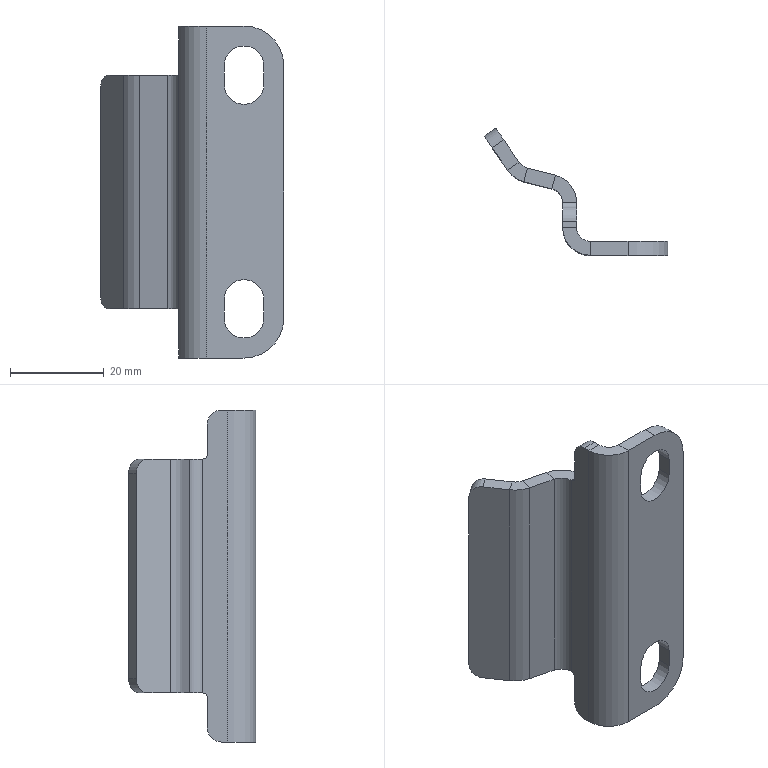Part | SolidWorks | features BaseBody 1 | 1 solid | 48 faces | box 39.243 x 27.212 x 71 mm | volume 9074 mm3 | plane 30 | cylinder 18 | commonest cylinder face diameters 6 x7 8.5 x4 12 x3 2 x2 17 x2
STEP:
#1=CARTESIAN_POINT('',(-4.25,0.,-27.));
#2=VERTEX_POINT('',#1);
#3=CARTESIAN_POINT('',(-4.25,0.,-23.));
#4=VERTEX_POINT('',#3);
#5=CARTESIAN_POINT('',(-4.25,0.,-27.));
#6=DIRECTION('',(0.,0.,1.));
#7=VECTOR('',#6,1000.);
#8=LINE('',#5,#7);
#9=EDGE_CURVE('',#2,#4,#8,.T.);
#10=ORIENTED_EDGE('',*,*,#9,.T.);
#11=CARTESIAN_POINT('',(4.25,0.,-23.));
#12=VERTEX_POINT('',#11);
#13=CARTESIAN_POINT('',(0.,0.,-23.));
#14=DIRECTION('',(0.,-1.,0.));
#15=DIRECTION('',(1.,0.,0.));
#16=AXIS2_PLACEMENT_3D('',#13,#14,#15);
#17=CIRCLE('',#16,4.25);
#18=EDGE_CURVE('',#12,#4,#17,.T.);
#19=ORIENTED_EDGE('',*,*,#18,.F.);
#20=CARTESIAN_POINT('',(4.25,0.,-27.));
#21=VERTEX_POINT('',#20);
#22=CARTESIAN_POINT('',(4.25,0.,-23.));
#23=DIRECTION('',(0.,0.,-1.));
#24=VECTOR('',#23,1000.);
#25=LINE('',#22,#24);
#26=EDGE_CURVE('',#12,#21,#25,.T.);
#27=ORIENTED_EDGE('',*,*,#26,.T.);
#28=CARTESIAN_POINT('',(0.,0.,-27.));
#29=DIRECTION('',(0.,-1.,0.));
#30=DIRECTION('',(-1.,0.,0.));
#31=AXIS2_PLACEMENT_3D('',#28,#29,#30);
#32=CIRCLE('',#31,4.25);
#33=EDGE_CURVE('',#2,#21,#32,.T.);
#34=ORIENTED_EDGE('',*,*,#33,.F.);
#35=EDGE_LOOP('',(#10,#19,#27,#34));
#36=FACE_BOUND('',#35,.T.);
#37=CARTESIAN_POINT('',(-4.25,0.,23.));
#38=VERTEX_POINT('',#37);
#39=CARTESIAN_POINT('',(4.25,0.,23.));
#40=VERTEX_POINT('',#39);
#41=CARTESIAN_POINT('',(0.,0.,23.));
#42=DIRECTION('',(0.,-1.,0.));
#43=DIRECTION('',(-1.,0.,0.));
#44=AXIS2_PLACEMENT_3D('',#41,#42,#43);
#45=CIRCLE('',#44,4.25);
#46=EDGE_CURVE('',#38,#40,#45,.T.);
#47=ORIENTED_EDGE('',*,*,#46,.F.);
#48=CARTESIAN_POINT('',(-4.25,0.,27.));
#49=VERTEX_POINT('',#48);
#50=CARTESIAN_POINT('',(-4.25,0.,23.));
#51=DIRECTION('',(0.,0.,1.));
#52=VECTOR('',#51,1000.);
#53=LINE('',#50,#52);
#54=EDGE_CURVE('',#38,#49,#53,.T.);
#55=ORIENTED_EDGE('',*,*,#54,.T.);
#56=CARTESIAN_POINT('',(4.25,0.,27.));
#57=VERTEX_POINT('',#56);
#58=CARTESIAN_POINT('',(0.,0.,27.));
#59=DIRECTION('',(0.,-1.,0.));
#60=DIRECTION('',(1.,0.,0.));
#61=AXIS2_PLACEMENT_3D('',#58,#59,#60);
#62=CIRCLE('',#61,4.25);
#63=EDGE_CURVE('',#57,#49,#62,.T.);
#64=ORIENTED_EDGE('',*,*,#63,.F.);
#65=CARTESIAN_POINT('',(4.25,0.,27.));
#66=DIRECTION('',(0.,0.,-1.));
#67=VECTOR('',#66,1000.);
#68=LINE('',#65,#67);
#69=EDGE_CURVE('',#57,#40,#68,.T.);
#70=ORIENTED_EDGE('',*,*,#69,.T.);
#71=EDGE_LOOP('',(#47,#55,#64,#70));
#72=FACE_BOUND('',#71,.T.);
#73=CARTESIAN_POINT('',(8.5,0.,27.));
#74=VERTEX_POINT('',#73);
#75=CARTESIAN_POINT('',(8.5,0.,-27.));
#76=VERTEX_POINT('',#75);
#77=CARTESIAN_POINT('',(8.5,0.,27.));
#78=DIRECTION('',(0.,0.,-1.));
#79=VECTOR('',#78,1000.);
#80=LINE('',#77,#79);
#81=EDGE_CURVE('',#74,#76,#80,.T.);
#82=ORIENTED_EDGE('',*,*,#81,.F.);
#83=CARTESIAN_POINT('',(0.,0.,35.5));
#84=VERTEX_POINT('',#83);
#85=CARTESIAN_POINT('',(0.,0.,27.));
#86=DIRECTION('',(0.,1.,0.));
#87=DIRECTION('',(0.,0.,1.));
#88=AXIS2_PLACEMENT_3D('',#85,#86,#87);
#89=CIRCLE('',#88,8.5);
#90=EDGE_CURVE('',#84,#74,#89,.T.);
#91=ORIENTED_EDGE('',*,*,#90,.F.);
#92=CARTESIAN_POINT('',(-8.,0.,35.5));
#93=VERTEX_POINT('',#92);
#94=CARTESIAN_POINT('',(0.,0.,35.5));
#95=DIRECTION('',(-1.,0.,0.));
#96=VECTOR('',#95,1000.);
#97=LINE('',#94,#96);
#98=EDGE_CURVE('',#84,#93,#97,.T.);
#99=ORIENTED_EDGE('',*,*,#98,.T.);
#100=CARTESIAN_POINT('',(-8.,0.,-35.5));
#101=VERTEX_POINT('',#100);
#102=CARTESIAN_POINT('',(-8.,0.,35.5));
#103=DIRECTION('',(0.,0.,-1.));
#104=VECTOR('',#103,1000.);
#105=LINE('',#102,#104);
#106=EDGE_CURVE('',#93,#101,#105,.T.);
#107=ORIENTED_EDGE('',*,*,#106,.T.);
#108=CARTESIAN_POINT('',(0.,0.,-35.5));
#109=VERTEX_POINT('',#108);
#110=CARTESIAN_POINT('',(0.,0.,-35.5));
#111=DIRECTION('',(-1.,0.,0.));
#112=VECTOR('',#111,1000.);
#113=LINE('',#110,#112);
#114=EDGE_CURVE('',#109,#101,#113,.T.);
#115=ORIENTED_EDGE('',*,*,#114,.F.);
#116=CARTESIAN_POINT('',(0.,0.,-27.));
#117=DIRECTION('',(0.,1.,0.));
#118=DIRECTION('',(1.,0.,0.));
#119=AXIS2_PLACEMENT_3D('',#116,#117,#118);
#120=CIRCLE('',#119,8.5);
#121=EDGE_CURVE('',#76,#109,#120,.T.);
#122=ORIENTED_EDGE('',*,*,#121,.F.);
#123=EDGE_LOOP('',(#82,#91,#99,#107,#115,#122));
#124=FACE_OUTER_BOUND('',#123,.T.);
#125=CARTESIAN_POINT('',(-11.,0.,-35.5));
#126=DIRECTION('',(0.,-1.,0.));
#127=DIRECTION('',(0.,0.,-1.));
#128=AXIS2_PLACEMENT_3D('',#125,#126,#127);
#129=PLANE('',#128);
#130=ADVANCED_FACE('',(#36,#72,#124),#129,.T.);
#131=CARTESIAN_POINT('',(0.,3.,-35.5));
#132=VERTEX_POINT('',#131);
#133=CARTESIAN_POINT('',(0.,3.,-35.5));
#134=DIRECTION('',(0.,-1.,0.));
#135=VECTOR('',#134,1000.);
#136=LINE('',#133,#135);
#137=EDGE_CURVE('',#132,#109,#136,.T.);
#138=ORIENTED_EDGE('',*,*,#137,.F.);
#139=CARTESIAN_POINT('',(8.5,3.,-27.));
#140=VERTEX_POINT('',#139);
#141=CARTESIAN_POINT('',(0.,3.,-27.));
#142=DIRECTION('',(0.,-1.,0.));
#143=DIRECTION('',(0.,0.,-1.));
#144=AXIS2_PLACEMENT_3D('',#141,#142,#143);
#145=CIRCLE('',#144,8.5);
#146=EDGE_CURVE('',#132,#140,#145,.T.);
#147=ORIENTED_EDGE('',*,*,#146,.T.);
#148=CARTESIAN_POINT('',(8.5,0.,-27.));
#149=DIRECTION('',(0.,1.,0.));
#150=VECTOR('',#149,1000.);
#151=LINE('',#148,#150);
#152=EDGE_CURVE('',#76,#140,#151,.T.);
#153=ORIENTED_EDGE('',*,*,#152,.F.);
#154=ORIENTED_EDGE('',*,*,#121,.T.);
#155=EDGE_LOOP('',(#138,#147,#153,#154));
#156=FACE_OUTER_BOUND('',#155,.T.);
#157=CARTESIAN_POINT('',(0.,1.5,-27.));
#158=DIRECTION('',(0.,-1.,0.));
#159=DIRECTION('',(0.,0.,-1.));
#160=AXIS2_PLACEMENT_3D('',#157,#158,#159);
#161=CYLINDRICAL_SURFACE('',#160,8.5);
#162=ADVANCED_FACE('',(#156),#161,.T.);
#163=ORIENTED_EDGE('',*,*,#152,.T.);
#164=CARTESIAN_POINT('',(8.5,3.,27.));
#165=VERTEX_POINT('',#164);
#166=CARTESIAN_POINT('',(8.5,3.,27.));
#167=DIRECTION('',(0.,0.,-1.));
#168=VECTOR('',#167,1000.);
#169=LINE('',#166,#168);
#170=EDGE_CURVE('',#165,#140,#169,.T.);
#171=ORIENTED_EDGE('',*,*,#170,.F.);
#172=CARTESIAN_POINT('',(8.5,3.,27.));
#173=DIRECTION('',(0.,-1.,0.));
#174=VECTOR('',#173,1000.);
#175=LINE('',#172,#174);
#176=EDGE_CURVE('',#165,#74,#175,.T.);
#177=ORIENTED_EDGE('',*,*,#176,.T.);
#178=ORIENTED_EDGE('',*,*,#81,.T.);
#179=EDGE_LOOP('',(#163,#171,#177,#178));
#180=FACE_OUTER_BOUND('',#179,.T.);
#181=CARTESIAN_POINT('',(8.5,1.5,0.));
#182=DIRECTION('',(1.,0.,0.));
#183=DIRECTION('',(0.,1.,0.));
#184=AXIS2_PLACEMENT_3D('',#181,#182,#183);
#185=PLANE('',#184);
#186=ADVANCED_FACE('',(#180),#185,.T.);
#187=ORIENTED_EDGE('',*,*,#176,.F.);
#188=CARTESIAN_POINT('',(0.,3.,35.5));
#189=VERTEX_POINT('',#188);
#190=CARTESIAN_POINT('',(0.,3.,27.));
#191=DIRECTION('',(0.,-1.,0.));
#192=DIRECTION('',(1.,0.,0.));
#193=AXIS2_PLACEMENT_3D('',#190,#191,#192);
#194=CIRCLE('',#193,8.5);
#195=EDGE_CURVE('',#165,#189,#194,.T.);
#196=ORIENTED_EDGE('',*,*,#195,.T.);
#197=CARTESIAN_POINT('',(0.,0.,35.5));
#198=DIRECTION('',(0.,1.,0.));
#199=VECTOR('',#198,1000.);
#200=LINE('',#197,#199);
#201=EDGE_CURVE('',#84,#189,#200,.T.);
#202=ORIENTED_EDGE('',*,*,#201,.F.);
#203=ORIENTED_EDGE('',*,*,#90,.T.);
#204=EDGE_LOOP('',(#187,#196,#202,#203));
#205=FACE_OUTER_BOUND('',#204,.T.);
#206=CARTESIAN_POINT('',(0.,1.5,27.));
#207=DIRECTION('',(0.,-1.,0.));
#208=DIRECTION('',(1.,0.,0.));
#209=AXIS2_PLACEMENT_3D('',#206,#207,#208);
#210=CYLINDRICAL_SURFACE('',#209,8.5);
#211=ADVANCED_FACE('',(#205),#210,.T.);
#212=ORIENTED_EDGE('',*,*,#201,.T.);
#213=CARTESIAN_POINT('',(-8.,3.,35.5));
#214=VERTEX_POINT('',#213);
#215=CARTESIAN_POINT('',(0.,3.,35.5));
#216=DIRECTION('',(-1.,0.,0.));
#217=VECTOR('',#216,1000.);
#218=LINE('',#215,#217);
#219=EDGE_CURVE('',#189,#214,#218,.T.);
#220=ORIENTED_EDGE('',*,*,#219,.T.);
#221=CARTESIAN_POINT('',(-8.,3.,35.5));
#222=DIRECTION('',(0.,-1.,0.));
#223=VECTOR('',#222,1000.);
#224=LINE('',#221,#223);
#225=EDGE_CURVE('',#214,#93,#224,.T.);
#226=ORIENTED_EDGE('',*,*,#225,.T.);
#227=ORIENTED_EDGE('',*,*,#98,.F.);
#228=EDGE_LOOP('',(#212,#220,#226,#227));
#229=FACE_OUTER_BOUND('',#228,.T.);
#230=CARTESIAN_POINT('',(-4.,1.5,35.5));
#231=DIRECTION('',(0.,0.,-1.));
#232=DIRECTION('',(-1.,0.,0.));
#233=AXIS2_PLACEMENT_3D('',#230,#231,#232);
#234=PLANE('',#233);
#235=ADVANCED_FACE('',(#229),#234,.F.);
#236=ORIENTED_EDGE('',*,*,#225,.F.);
#237=CARTESIAN_POINT('',(-11.,6.,35.5));
#238=VERTEX_POINT('',#237);
#239=CARTESIAN_POINT('',(-8.,6.,35.5));
#240=DIRECTION('',(0.,0.,1.));
#241=DIRECTION('',(-1.,0.,0.));
#242=AXIS2_PLACEMENT_3D('',#239,#240,#241);
#243=CIRCLE('',#242,3.);
#244=EDGE_CURVE('',#238,#214,#243,.T.);
#245=ORIENTED_EDGE('',*,*,#244,.F.);
#246=CARTESIAN_POINT('',(-14.,6.,35.5));
#247=VERTEX_POINT('',#246);
#248=CARTESIAN_POINT('',(-11.,6.,35.5));
#249=DIRECTION('',(-1.,0.,0.));
#250=VECTOR('',#249,1000.);
#251=LINE('',#248,#250);
#252=EDGE_CURVE('',#238,#247,#251,.T.);
#253=ORIENTED_EDGE('',*,*,#252,.T.);
#254=CARTESIAN_POINT('',(-8.,6.,35.5));
#255=DIRECTION('',(0.,0.,-1.));
#256=DIRECTION('',(0.,-1.,0.));
#257=AXIS2_PLACEMENT_3D('',#254,#255,#256);
#258=CIRCLE('',#257,6.);
#259=EDGE_CURVE('',#93,#247,#258,.T.);
#260=ORIENTED_EDGE('',*,*,#259,.F.);
#261=EDGE_LOOP('',(#236,#245,#253,#260));
#262=FACE_OUTER_BOUND('',#261,.T.);
#263=CARTESIAN_POINT('',(-11.182,2.818,35.5));
#264=DIRECTION('',(0.,0.,1.));
#265=DIRECTION('',(1.,0.,0.));
#266=AXIS2_PLACEMENT_3D('',#263,#264,#265);
#267=PLANE('',#266);
#268=ADVANCED_FACE('',(#262),#267,.T.);
#269=CARTESIAN_POINT('',(-14.,6.,-35.5));
#270=VERTEX_POINT('',#269);
#271=CARTESIAN_POINT('',(-14.,6.,-35.5));
#272=DIRECTION('',(0.,0.,1.));
#273=VECTOR('',#272,1000.);
#274=LINE('',#271,#273);
#275=EDGE_CURVE('',#270,#247,#274,.T.);
#276=ORIENTED_EDGE('',*,*,#275,.F.);
#277=CARTESIAN_POINT('',(-8.,6.,-35.5));
#278=DIRECTION('',(0.,0.,1.));
#279=DIRECTION('',(-1.,0.,0.));
#280=AXIS2_PLACEMENT_3D('',#277,#278,#279);
#281=CIRCLE('',#280,6.);
#282=EDGE_CURVE('',#270,#101,#281,.T.);
#283=ORIENTED_EDGE('',*,*,#282,.T.);
#284=ORIENTED_EDGE('',*,*,#106,.F.);
#285=ORIENTED_EDGE('',*,*,#259,.T.);
#286=EDGE_LOOP('',(#276,#283,#284,#285));
#287=FACE_OUTER_BOUND('',#286,.T.);
#288=CARTESIAN_POINT('',(-8.,6.,137.27));
#289=DIRECTION('',(0.,0.,-1.));
#290=DIRECTION('',(0.,-1.,0.));
#291=AXIS2_PLACEMENT_3D('',#288,#289,#290);
#292=CYLINDRICAL_SURFACE('',#291,6.);
#293=ADVANCED_FACE('',(#287),#292,.T.);
#294=CARTESIAN_POINT('',(-11.,6.,-35.5));
#295=VERTEX_POINT('',#294);
#296=CARTESIAN_POINT('',(-11.,6.,-35.5));
#297=DIRECTION('',(-1.,0.,0.));
#298=VECTOR('',#297,1000.);
#299=LINE('',#296,#298);
#300=EDGE_CURVE('',#295,#270,#299,.T.);
#301=ORIENTED_EDGE('',*,*,#300,.F.);
#302=CARTESIAN_POINT('',(-8.,3.,-35.5));
#303=VERTEX_POINT('',#302);
#304=CARTESIAN_POINT('',(-8.,6.,-35.5));
#305=DIRECTION('',(0.,0.,-1.));
#306=DIRECTION('',(0.,-1.,0.));
#307=AXIS2_PLACEMENT_3D('',#304,#305,#306);
#308=CIRCLE('',#307,3.);
#309=EDGE_CURVE('',#303,#295,#308,.T.);
#310=ORIENTED_EDGE('',*,*,#309,.F.);
#311=CARTESIAN_POINT('',(-8.,3.,-35.5));
#312=DIRECTION('',(0.,-1.,0.));
#313=VECTOR('',#312,1000.);
#314=LINE('',#311,#313);
#315=EDGE_CURVE('',#303,#101,#314,.T.);
#316=ORIENTED_EDGE('',*,*,#315,.T.);
#317=ORIENTED_EDGE('',*,*,#282,.F.);
#318=EDGE_LOOP('',(#301,#310,#316,#317));
#319=FACE_OUTER_BOUND('',#318,.T.);
#320=CARTESIAN_POINT('',(-11.182,2.818,-35.5));
#321=DIRECTION('',(0.,0.,1.));
#322=DIRECTION('',(1.,0.,0.));
#323=AXIS2_PLACEMENT_3D('',#320,#321,#322);
#324=PLANE('',#323);
#325=ADVANCED_FACE('',(#319),#324,.F.);
#326=ORIENTED_EDGE('',*,*,#315,.F.);
#327=CARTESIAN_POINT('',(0.,3.,-35.5));
#328=DIRECTION('',(-1.,0.,0.));
#329=VECTOR('',#328,1000.);
#330=LINE('',#327,#329);
#331=EDGE_CURVE('',#132,#303,#330,.T.);
#332=ORIENTED_EDGE('',*,*,#331,.F.);
#333=ORIENTED_EDGE('',*,*,#137,.T.);
#334=ORIENTED_EDGE('',*,*,#114,.T.);
#335=EDGE_LOOP('',(#326,#332,#333,#334));
#336=FACE_OUTER_BOUND('',#335,.T.);
#337=CARTESIAN_POINT('',(-4.,1.5,-35.5));
#338=DIRECTION('',(0.,0.,-1.));
#339=DIRECTION('',(0.,-1.,0.));
#340=AXIS2_PLACEMENT_3D('',#337,#338,#339);
#341=PLANE('',#340);
#342=ADVANCED_FACE('',(#336),#341,.T.);
#343=CARTESIAN_POINT('',(4.25,3.,-23.));
#344=VERTEX_POINT('',#343);
#345=CARTESIAN_POINT('',(4.25,3.,-27.));
#346=VERTEX_POINT('',#345);
#347=CARTESIAN_POINT('',(4.25,3.,-23.));
#348=DIRECTION('',(0.,0.,-1.));
#349=VECTOR('',#348,1000.);
#350=LINE('',#347,#349);
#351=EDGE_CURVE('',#344,#346,#350,.T.);
#352=ORIENTED_EDGE('',*,*,#351,.F.);
#353=CARTESIAN_POINT('',(-4.25,3.,-23.));
#354=VERTEX_POINT('',#353);
#355=CARTESIAN_POINT('',(0.,3.,-23.));
#356=DIRECTION('',(0.,1.,0.));
#357=DIRECTION('',(-1.,0.,0.));
#358=AXIS2_PLACEMENT_3D('',#355,#356,#357);
#359=CIRCLE('',#358,4.25);
#360=EDGE_CURVE('',#354,#344,#359,.T.);
#361=ORIENTED_EDGE('',*,*,#360,.F.);
#362=CARTESIAN_POINT('',(-4.25,3.,-27.));
#363=VERTEX_POINT('',#362);
#364=CARTESIAN_POINT('',(-4.25,3.,-27.));
#365=DIRECTION('',(0.,0.,1.));
#366=VECTOR('',#365,1000.);
#367=LINE('',#364,#366);
#368=EDGE_CURVE('',#363,#354,#367,.T.);
#369=ORIENTED_EDGE('',*,*,#368,.F.);
#370=CARTESIAN_POINT('',(0.,3.,-27.));
#371=DIRECTION('',(0.,1.,0.));
#372=DIRECTION('',(1.,0.,0.));
#373=AXIS2_PLACEMENT_3D('',#370,#371,#372);
#374=CIRCLE('',#373,4.25);
#375=EDGE_CURVE('',#346,#363,#374,.T.);
#376=ORIENTED_EDGE('',*,*,#375,.F.);
#377=EDGE_LOOP('',(#352,#361,#369,#376));
#378=FACE_BOUND('',#377,.T.);
#379=CARTESIAN_POINT('',(-4.25,3.,27.));
#380=VERTEX_POINT('',#379);
#381=CARTESIAN_POINT('',(4.25,3.,27.));
#382=VERTEX_POINT('',#381);
#383=CARTESIAN_POINT('',(0.,3.,27.));
#384=DIRECTION('',(0.,1.,0.));
#385=DIRECTION('',(-1.,0.,0.));
#386=AXIS2_PLACEMENT_3D('',#383,#384,#385);
#387=CIRCLE('',#386,4.25);
#388=EDGE_CURVE('',#380,#382,#387,.T.);
#389=ORIENTED_EDGE('',*,*,#388,.F.);
#390=CARTESIAN_POINT('',(-4.25,3.,23.));
#391=VERTEX_POINT('',#390);
#392=CARTESIAN_POINT('',(-4.25,3.,23.));
#393=DIRECTION('',(0.,0.,1.));
#394=VECTOR('',#393,1000.);
#395=LINE('',#392,#394);
#396=EDGE_CURVE('',#391,#380,#395,.T.);
#397=ORIENTED_EDGE('',*,*,#396,.F.);
#398=CARTESIAN_POINT('',(4.25,3.,23.));
#399=VERTEX_POINT('',#398);
#400=CARTESIAN_POINT('',(0.,3.,23.));
#401=DIRECTION('',(0.,1.,0.));
#402=DIRECTION('',(1.,0.,0.));
#403=AXIS2_PLACEMENT_3D('',#400,#401,#402);
#404=CIRCLE('',#403,4.25);
#405=EDGE_CURVE('',#399,#391,#404,.T.);
#406=ORIENTED_EDGE('',*,*,#405,.F.);
#407=CARTESIAN_POINT('',(4.25,3.,27.));
#408=DIRECTION('',(0.,0.,-1.));
#409=VECTOR('',#408,1000.);
#410=LINE('',#407,#409);
#411=EDGE_CURVE('',#382,#399,#410,.T.);
#412=ORIENTED_EDGE('',*,*,#411,.F.);
#413=EDGE_LOOP('',(#389,#397,#406,#412));
#414=FACE_BOUND('',#413,.T.);
#415=ORIENTED_EDGE('',*,*,#331,.T.);
#416=CARTESIAN_POINT('',(-8.,3.,-35.5));
#417=DIRECTION('',(0.,0.,1.));
#418=VECTOR('',#417,1000.);
#419=LINE('',#416,#418);
#420=EDGE_CURVE('',#303,#214,#419,.T.);
#421=ORIENTED_EDGE('',*,*,#420,.T.);
#422=ORIENTED_EDGE('',*,*,#219,.F.);
#423=ORIENTED_EDGE('',*,*,#195,.F.);
#424=ORIENTED_EDGE('',*,*,#170,.T.);
#425=ORIENTED_EDGE('',*,*,#146,.F.);
#426=EDGE_LOOP('',(#415,#421,#422,#423,#424,#425));
#427=FACE_OUTER_BOUND('',#426,.T.);
#428=CARTESIAN_POINT('',(-11.,3.,-35.5));
#429=DIRECTION('',(0.,-1.,0.));
#430=DIRECTION('',(0.,0.,-1.));
#431=AXIS2_PLACEMENT_3D('',#428,#429,#430);
#432=PLANE('',#431);
#433=ADVANCED_FACE('',(#378,#414,#427),#432,.F.);
#434=ORIENTED_EDGE('',*,*,#420,.F.);
#435=ORIENTED_EDGE('',*,*,#309,.T.);
#436=CARTESIAN_POINT('',(-11.,6.,35.5));
#437=DIRECTION('',(0.,0.,-1.));
#438=VECTOR('',#437,1000.);
#439=LINE('',#436,#438);
#440=EDGE_CURVE('',#238,#295,#439,.T.);
#441=ORIENTED_EDGE('',*,*,#440,.F.);
#442=ORIENTED_EDGE('',*,*,#244,.T.);
#443=EDGE_LOOP('',(#434,#435,#441,#442));
#444=FACE_OUTER_BOUND('',#443,.T.);
#445=CARTESIAN_POINT('',(-8.,6.,137.27));
#446=DIRECTION('',(0.,0.,-1.));
#447=DIRECTION('',(0.,-1.,0.));
#448=AXIS2_PLACEMENT_3D('',#445,#446,#447);
#449=CYLINDRICAL_SURFACE('',#448,3.);
#450=ADVANCED_FACE('',(#444),#449,.F.);
#451=CARTESIAN_POINT('',(-11.,11.325,-25.));
#452=VERTEX_POINT('',#451);
#453=CARTESIAN_POINT('',(-11.,10.325,-26.));
#454=VERTEX_POINT('',#453);
#455=CARTESIAN_POINT('',(-11.,11.325,-26.));
#456=DIRECTION('',(1.,0.,0.));
#457=DIRECTION('',(0.,0.,1.));
#458=AXIS2_PLACEMENT_3D('',#455,#456,#457);
#459=CIRCLE('',#458,1.);
#460=EDGE_CURVE('',#452,#454,#459,.T.);
#461=ORIENTED_EDGE('',*,*,#460,.F.);
#462=CARTESIAN_POINT('',(-11.,11.325,25.));
#463=VERTEX_POINT('',#462);
#464=CARTESIAN_POINT('',(-11.,11.325,-25.));
#465=DIRECTION('',(0.,0.,1.));
#466=VECTOR('',#465,1000.);
#467=LINE('',#464,#466);
#468=EDGE_CURVE('',#452,#463,#467,.T.);
#469=ORIENTED_EDGE('',*,*,#468,.T.);
#470=CARTESIAN_POINT('',(-11.,10.325,26.));
#471=VERTEX_POINT('',#470);
#472=CARTESIAN_POINT('',(-11.,11.325,26.));
#473=DIRECTION('',(1.,0.,0.));
#474=DIRECTION('',(0.,-1.,0.));
#475=AXIS2_PLACEMENT_3D('',#472,#473,#474);
#476=CIRCLE('',#475,1.);
#477=EDGE_CURVE('',#471,#463,#476,.T.);
#478=ORIENTED_EDGE('',*,*,#477,.F.);
#479=CARTESIAN_POINT('',(-11.,10.325,32.5));
#480=VERTEX_POINT('',#479);
#481=CARTESIAN_POINT('',(-11.,10.325,26.));
#482=DIRECTION('',(0.,0.,1.));
#483=VECTOR('',#482,1000.);
#484=LINE('',#481,#483);
#485=EDGE_CURVE('',#471,#480,#484,.T.);
#486=ORIENTED_EDGE('',*,*,#485,.T.);
#487=CARTESIAN_POINT('',(-11.,7.325,35.5));
#488=VERTEX_POINT('',#487);
#489=CARTESIAN_POINT('',(-11.,7.325,32.5));
#490=DIRECTION('',(-1.,0.,0.));
#491=DIRECTION('',(0.,0.,1.));
#492=AXIS2_PLACEMENT_3D('',#489,#490,#491);
#493=CIRCLE('',#492,3.);
#494=EDGE_CURVE('',#488,#480,#493,.T.);
#495=ORIENTED_EDGE('',*,*,#494,.F.);
#496=CARTESIAN_POINT('',(-11.,6.,35.5));
#497=DIRECTION('',(0.,1.,0.));
#498=VECTOR('',#497,1000.);
#499=LINE('',#496,#498);
#500=EDGE_CURVE('',#238,#488,#499,.T.);
#501=ORIENTED_EDGE('',*,*,#500,.F.);
#502=ORIENTED_EDGE('',*,*,#440,.T.);
#503=CARTESIAN_POINT('',(-11.,7.325,-35.5));
#504=VERTEX_POINT('',#503);
#505=CARTESIAN_POINT('',(-11.,6.,-35.5));
#506=DIRECTION('',(0.,1.,0.));
#507=VECTOR('',#506,1000.);
#508=LINE('',#505,#507);
#509=EDGE_CURVE('',#295,#504,#508,.T.);
#510=ORIENTED_EDGE('',*,*,#509,.T.);
#511=CARTESIAN_POINT('',(-11.,10.325,-32.5));
#512=VERTEX_POINT('',#511);
#513=CARTESIAN_POINT('',(-11.,7.325,-32.5));
#514=DIRECTION('',(-1.,0.,0.));
#515=DIRECTION('',(0.,1.,0.));
#516=AXIS2_PLACEMENT_3D('',#513,#514,#515);
#517=CIRCLE('',#516,3.);
#518=EDGE_CURVE('',#512,#504,#517,.T.);
#519=ORIENTED_EDGE('',*,*,#518,.F.);
#520=CARTESIAN_POINT('',(-11.,10.325,-26.));
#521=DIRECTION('',(0.,0.,-1.));
#522=VECTOR('',#521,1000.);
#523=LINE('',#520,#522);
#524=EDGE_CURVE('',#454,#512,#523,.T.);
#525=ORIENTED_EDGE('',*,*,#524,.F.);
#526=EDGE_LOOP('',(#461,#469,#478,#486,#495,#501,#502,#510,#519,#525));
#527=FACE_OUTER_BOUND('',#526,.T.);
#528=CARTESIAN_POINT('',(-11.,16.,-35.5));
#529=DIRECTION('',(-1.,0.,0.));
#530=DIRECTION('',(0.,0.,1.));
#531=AXIS2_PLACEMENT_3D('',#528,#529,#530);
#532=PLANE('',#531);
#533=ADVANCED_FACE('',(#527),#532,.F.);
#534=CARTESIAN_POINT('',(-14.,10.325,-26.));
#535=VERTEX_POINT('',#534);
#536=CARTESIAN_POINT('',(-14.,10.325,-26.));
#537=DIRECTION('',(1.,0.,0.));
#538=VECTOR('',#537,1000.);
#539=LINE('',#536,#538);
#540=EDGE_CURVE('',#535,#454,#539,.T.);
#541=ORIENTED_EDGE('',*,*,#540,.T.);
#542=ORIENTED_EDGE('',*,*,#524,.T.);
#543=CARTESIAN_POINT('',(-14.,10.325,-32.5));
#544=VERTEX_POINT('',#543);
#545=CARTESIAN_POINT('',(-11.,10.325,-32.5));
#546=DIRECTION('',(-1.,0.,0.));
#547=VECTOR('',#546,1000.);
#548=LINE('',#545,#547);
#549=EDGE_CURVE('',#512,#544,#548,.T.);
#550=ORIENTED_EDGE('',*,*,#549,.T.);
#551=CARTESIAN_POINT('',(-14.,10.325,-26.));
#552=DIRECTION('',(0.,0.,-1.));
#553=VECTOR('',#552,1000.);
#554=LINE('',#551,#553);
#555=EDGE_CURVE('',#535,#544,#554,.T.);
#556=ORIENTED_EDGE('',*,*,#555,.F.);
#557=EDGE_LOOP('',(#541,#542,#550,#556));
#558=FACE_OUTER_BOUND('',#557,.T.);
#559=CARTESIAN_POINT('',(-12.5,10.325,-29.25));
#560=DIRECTION('',(0.,-1.,0.));
#561=DIRECTION('',(0.,0.,-1.));
#562=AXIS2_PLACEMENT_3D('',#559,#560,#561);
#563=PLANE('',#562);
#564=ADVANCED_FACE('',(#558),#563,.F.);
#565=CARTESIAN_POINT('',(-14.,7.325,-35.5));
#566=VERTEX_POINT('',#565);
#567=CARTESIAN_POINT('',(-14.,7.325,-32.5));
#568=DIRECTION('',(1.,0.,0.));
#569=DIRECTION('',(0.,0.,-1.));
#570=AXIS2_PLACEMENT_3D('',#567,#568,#569);
#571=CIRCLE('',#570,3.);
#572=EDGE_CURVE('',#566,#544,#571,.T.);
#573=ORIENTED_EDGE('',*,*,#572,.F.);
#574=CARTESIAN_POINT('',(-14.,6.,-35.5));
#575=DIRECTION('',(0.,1.,0.));
#576=VECTOR('',#575,1000.);
#577=LINE('',#574,#576);
#578=EDGE_CURVE('',#270,#566,#577,.T.);
#579=ORIENTED_EDGE('',*,*,#578,.F.);
#580=ORIENTED_EDGE('',*,*,#275,.T.);
#581=CARTESIAN_POINT('',(-14.,7.325,35.5));
#582=VERTEX_POINT('',#581);
#583=CARTESIAN_POINT('',(-14.,6.,35.5));
#584=DIRECTION('',(0.,1.,0.));
#585=VECTOR('',#584,1000.);
#586=LINE('',#583,#585);
#587=EDGE_CURVE('',#247,#582,#586,.T.);
#588=ORIENTED_EDGE('',*,*,#587,.T.);
#589=CARTESIAN_POINT('',(-14.,10.325,32.5));
#590=VERTEX_POINT('',#589);
#591=CARTESIAN_POINT('',(-14.,7.325,32.5));
#592=DIRECTION('',(1.,0.,0.));
#593=DIRECTION('',(0.,1.,0.));
#594=AXIS2_PLACEMENT_3D('',#591,#592,#593);
#595=CIRCLE('',#594,3.);
#596=EDGE_CURVE('',#590,#582,#595,.T.);
#597=ORIENTED_EDGE('',*,*,#596,.F.);
#598=CARTESIAN_POINT('',(-14.,10.325,26.));
#599=VERTEX_POINT('',#598);
#600=CARTESIAN_POINT('',(-14.,10.325,26.));
#601=DIRECTION('',(0.,0.,1.));
#602=VECTOR('',#601,1000.);
#603=LINE('',#600,#602);
#604=EDGE_CURVE('',#599,#590,#603,.T.);
#605=ORIENTED_EDGE('',*,*,#604,.F.);
#606=CARTESIAN_POINT('',(-14.,11.325,25.));
#607=VERTEX_POINT('',#606);
#608=CARTESIAN_POINT('',(-14.,11.325,26.));
#609=DIRECTION('',(-1.,0.,0.));
#610=DIRECTION('',(0.,0.,-1.));
#611=AXIS2_PLACEMENT_3D('',#608,#609,#610);
#612=CIRCLE('',#611,1.);
#613=EDGE_CURVE('',#607,#599,#612,.T.);
#614=ORIENTED_EDGE('',*,*,#613,.F.);
#615=CARTESIAN_POINT('',(-14.,11.325,-25.));
#616=VERTEX_POINT('',#615);
#617=CARTESIAN_POINT('',(-14.,11.325,25.));
#618=DIRECTION('',(0.,0.,-1.));
#619=VECTOR('',#618,1000.);
#620=LINE('',#617,#619);
#621=EDGE_CURVE('',#607,#616,#620,.T.);
#622=ORIENTED_EDGE('',*,*,#621,.T.);
#623=CARTESIAN_POINT('',(-14.,11.325,-26.));
#624=DIRECTION('',(-1.,0.,0.));
#625=DIRECTION('',(0.,-1.,0.));
#626=AXIS2_PLACEMENT_3D('',#623,#624,#625);
#627=CIRCLE('',#626,1.);
#628=EDGE_CURVE('',#535,#616,#627,.T.);
#629=ORIENTED_EDGE('',*,*,#628,.F.);
#630=ORIENTED_EDGE('',*,*,#555,.T.);
#631=EDGE_LOOP('',(#573,#579,#580,#588,#597,#605,#614,#622,#629,#630));
#632=FACE_OUTER_BOUND('',#631,.T.);
#633=CARTESIAN_POINT('',(-14.,16.,-35.5));
#634=DIRECTION('',(-1.,0.,0.));
#635=DIRECTION('',(0.,0.,1.));
#636=AXIS2_PLACEMENT_3D('',#633,#634,#635);
#637=PLANE('',#636);
#638=ADVANCED_FACE('',(#632),#637,.T.);
#639=CARTESIAN_POINT('',(-11.,11.325,-25.));
#640=DIRECTION('',(-1.,0.,0.));
#641=VECTOR('',#640,1000.);
#642=LINE('',#639,#641);
#643=EDGE_CURVE('',#452,#616,#642,.T.);
#644=ORIENTED_EDGE('',*,*,#643,.F.);
#645=ORIENTED_EDGE('',*,*,#460,.T.);
#646=ORIENTED_EDGE('',*,*,#540,.F.);
#647=ORIENTED_EDGE('',*,*,#628,.T.);
#648=EDGE_LOOP('',(#644,#645,#646,#647));
#649=FACE_OUTER_BOUND('',#648,.T.);
#650=CARTESIAN_POINT('',(-12.5,11.325,-26.));
#651=DIRECTION('',(1.,0.,0.));
#652=DIRECTION('',(0.,0.,1.));
#653=AXIS2_PLACEMENT_3D('',#650,#651,#652);
#654=CYLINDRICAL_SURFACE('',#653,1.);
#655=ADVANCED_FACE('',(#649),#654,.F.);
#656=CARTESIAN_POINT('',(-15.534,17.143,-25.));
#657=VERTEX_POINT('',#656);
#658=CARTESIAN_POINT('',(-16.267,14.234,-25.));
#659=VERTEX_POINT('',#658);
#660=CARTESIAN_POINT('',(-15.534,17.143,-25.));
#661=DIRECTION('',(-0.2444,-0.9697,0.));
#662=VECTOR('',#661,1000.);
#663=LINE('',#660,#662);
#664=EDGE_CURVE('',#657,#659,#663,.T.);
#665=ORIENTED_EDGE('',*,*,#664,.F.);
#666=CARTESIAN_POINT('',(-17.,11.325,-25.));
#667=DIRECTION('',(0.,0.,1.));
#668=DIRECTION('',(1.,0.,0.));
#669=AXIS2_PLACEMENT_3D('',#666,#667,#668);
#670=CIRCLE('',#669,6.);
#671=EDGE_CURVE('',#452,#657,#670,.T.);
#672=ORIENTED_EDGE('',*,*,#671,.F.);
#673=ORIENTED_EDGE('',*,*,#643,.T.);
#674=CARTESIAN_POINT('',(-17.,11.325,-25.));
#675=DIRECTION('',(0.,0.,-1.));
#676=DIRECTION('',(0.2444,0.9697,0.));
#677=AXIS2_PLACEMENT_3D('',#674,#675,#676);
#678=CIRCLE('',#677,3.);
#679=EDGE_CURVE('',#659,#616,#678,.T.);
#680=ORIENTED_EDGE('',*,*,#679,.F.);
#681=EDGE_LOOP('',(#665,#672,#673,#680));
#682=FACE_OUTER_BOUND('',#681,.T.);
#683=CARTESIAN_POINT('',(-13.45,14.091,-25.));
#684=DIRECTION('',(0.,0.,1.));
#685=DIRECTION('',(1.,0.,0.));
#686=AXIS2_PLACEMENT_3D('',#683,#684,#685);
#687=PLANE('',#686);
#688=ADVANCED_FACE('',(#682),#687,.F.);
#689=CARTESIAN_POINT('',(-16.267,14.234,25.));
#690=VERTEX_POINT('',#689);
#691=CARTESIAN_POINT('',(-16.267,14.234,-25.));
#692=DIRECTION('',(0.,0.,1.));
#693=VECTOR('',#692,1000.);
#694=LINE('',#691,#693);
#695=EDGE_CURVE('',#659,#690,#694,.T.);
#696=ORIENTED_EDGE('',*,*,#695,.F.);
#697=ORIENTED_EDGE('',*,*,#679,.T.);
#698=ORIENTED_EDGE('',*,*,#621,.F.);
#699=CARTESIAN_POINT('',(-17.,11.325,25.));
#700=DIRECTION('',(0.,0.,1.));
#701=DIRECTION('',(1.,0.,0.));
#702=AXIS2_PLACEMENT_3D('',#699,#700,#701);
#703=CIRCLE('',#702,3.);
#704=EDGE_CURVE('',#607,#690,#703,.T.);
#705=ORIENTED_EDGE('',*,*,#704,.T.);
#706=EDGE_LOOP('',(#696,#697,#698,#705));
#707=FACE_OUTER_BOUND('',#706,.T.);
#708=CARTESIAN_POINT('',(-17.,11.325,-133.27));
#709=DIRECTION('',(0.,0.,1.));
#710=DIRECTION('',(1.,0.,0.));
#711=AXIS2_PLACEMENT_3D('',#708,#709,#710);
#712=CYLINDRICAL_SURFACE('',#711,3.);
#713=ADVANCED_FACE('',(#707),#712,.F.);
#714=CARTESIAN_POINT('',(-14.,11.325,25.));
#715=DIRECTION('',(1.,0.,0.));
#716=VECTOR('',#715,1000.);
#717=LINE('',#714,#716);
#718=EDGE_CURVE('',#607,#463,#717,.T.);
#719=ORIENTED_EDGE('',*,*,#718,.T.);
#720=CARTESIAN_POINT('',(-15.534,17.143,25.));
#721=VERTEX_POINT('',#720);
#722=CARTESIAN_POINT('',(-17.,11.325,25.));
#723=DIRECTION('',(0.,0.,-1.));
#724=DIRECTION('',(0.2444,0.9697,0.));
#725=AXIS2_PLACEMENT_3D('',#722,#723,#724);
#726=CIRCLE('',#725,6.);
#727=EDGE_CURVE('',#721,#463,#726,.T.);
#728=ORIENTED_EDGE('',*,*,#727,.F.);
#729=CARTESIAN_POINT('',(-16.267,14.234,25.));
#730=DIRECTION('',(0.2444,0.9697,0.));
#731=VECTOR('',#730,1000.);
#732=LINE('',#729,#731);
#733=EDGE_CURVE('',#690,#721,#732,.T.);
#734=ORIENTED_EDGE('',*,*,#733,.F.);
#735=ORIENTED_EDGE('',*,*,#704,.F.);
#736=EDGE_LOOP('',(#719,#728,#734,#735));
#737=FACE_OUTER_BOUND('',#736,.T.);
#738=CARTESIAN_POINT('',(-13.45,14.091,25.));
#739=DIRECTION('',(0.,0.,1.));
#740=DIRECTION('',(1.,0.,0.));
#741=AXIS2_PLACEMENT_3D('',#738,#739,#740);
#742=PLANE('',#741);
#743=ADVANCED_FACE('',(#737),#742,.T.);
#744=ORIENTED_EDGE('',*,*,#733,.T.);
#745=CARTESIAN_POINT('',(-21.539,18.656,25.));
#746=VERTEX_POINT('',#745);
#747=CARTESIAN_POINT('',(-15.534,17.143,25.));
#748=DIRECTION('',(-0.9697,0.2444,0.));
#749=VECTOR('',#748,1000.);
#750=LINE('',#747,#749);
#751=EDGE_CURVE('',#721,#746,#750,.T.);
#752=ORIENTED_EDGE('',*,*,#751,.T.);
#753=CARTESIAN_POINT('',(-22.272,15.747,25.));
#754=VERTEX_POINT('',#753);
#755=CARTESIAN_POINT('',(-21.539,18.656,25.));
#756=DIRECTION('',(-0.2444,-0.9697,0.));
#757=VECTOR('',#756,1000.);
#758=LINE('',#755,#757);
#759=EDGE_CURVE('',#746,#754,#758,.T.);
#760=ORIENTED_EDGE('',*,*,#759,.T.);
#761=CARTESIAN_POINT('',(-16.267,14.234,25.));
#762=DIRECTION('',(-0.9697,0.2444,0.));
#763=VECTOR('',#762,1000.);
#764=LINE('',#761,#763);
#765=EDGE_CURVE('',#690,#754,#764,.T.);
#766=ORIENTED_EDGE('',*,*,#765,.F.);
#767=EDGE_LOOP('',(#744,#752,#760,#766));
#768=FACE_OUTER_BOUND('',#767,.T.);
#769=CARTESIAN_POINT('',(-18.903,16.445,25.));
#770=DIRECTION('',(0.,0.,-1.));
#771=DIRECTION('',(0.,-1.,0.));
#772=AXIS2_PLACEMENT_3D('',#769,#770,#771);
#773=PLANE('',#772);
#774=ADVANCED_FACE('',(#768),#773,.F.);
#775=CARTESIAN_POINT('',(-22.272,15.747,-25.));
#776=VERTEX_POINT('',#775);
#777=CARTESIAN_POINT('',(-22.272,15.747,25.));
#778=DIRECTION('',(0.,0.,-1.));
#779=VECTOR('',#778,1000.);
#780=LINE('',#777,#779);
#781=EDGE_CURVE('',#754,#776,#780,.T.);
#782=ORIENTED_EDGE('',*,*,#781,.T.);
#783=CARTESIAN_POINT('',(-16.267,14.234,-25.));
#784=DIRECTION('',(-0.9697,0.2444,0.));
#785=VECTOR('',#784,1000.);
#786=LINE('',#783,#785);
#787=EDGE_CURVE('',#659,#776,#786,.T.);
#788=ORIENTED_EDGE('',*,*,#787,.F.);
#789=ORIENTED_EDGE('',*,*,#695,.T.);
#790=ORIENTED_EDGE('',*,*,#765,.T.);
#791=EDGE_LOOP('',(#782,#788,#789,#790));
#792=FACE_OUTER_BOUND('',#791,.T.);
#793=CARTESIAN_POINT('',(-23.38,16.027,-35.5));
#794=DIRECTION('',(-0.2444,-0.9697,0.));
#795=DIRECTION('',(-0.9697,0.2444,0.));
#796=AXIS2_PLACEMENT_3D('',#793,#794,#795);
#797=PLANE('',#796);
#798=ADVANCED_FACE('',(#792),#797,.T.);
#799=CARTESIAN_POINT('',(-21.539,18.656,-25.));
#800=VERTEX_POINT('',#799);
#801=CARTESIAN_POINT('',(-21.539,18.656,-25.));
#802=DIRECTION('',(-0.2444,-0.9697,0.));
#803=VECTOR('',#802,1000.);
#804=LINE('',#801,#803);
#805=EDGE_CURVE('',#800,#776,#804,.T.);
#806=ORIENTED_EDGE('',*,*,#805,.F.);
#807=CARTESIAN_POINT('',(-15.534,17.143,-25.));
#808=DIRECTION('',(-0.9697,0.2444,0.));
#809=VECTOR('',#808,1000.);
#810=LINE('',#807,#809);
#811=EDGE_CURVE('',#657,#800,#810,.T.);
#812=ORIENTED_EDGE('',*,*,#811,.F.);
#813=ORIENTED_EDGE('',*,*,#664,.T.);
#814=ORIENTED_EDGE('',*,*,#787,.T.);
#815=EDGE_LOOP('',(#806,#812,#813,#814));
#816=FACE_OUTER_BOUND('',#815,.T.);
#817=CARTESIAN_POINT('',(-18.903,16.445,-25.));
#818=DIRECTION('',(0.,0.,-1.));
#819=DIRECTION('',(0.,-1.,0.));
#820=AXIS2_PLACEMENT_3D('',#817,#818,#819);
#821=PLANE('',#820);
#822=ADVANCED_FACE('',(#816),#821,.T.);
#823=CARTESIAN_POINT('',(-15.534,17.143,25.));
#824=DIRECTION('',(0.,0.,-1.));
#825=VECTOR('',#824,1000.);
#826=LINE('',#823,#825);
#827=EDGE_CURVE('',#721,#657,#826,.T.);
#828=ORIENTED_EDGE('',*,*,#827,.T.);
#829=ORIENTED_EDGE('',*,*,#811,.T.);
#830=CARTESIAN_POINT('',(-21.539,18.656,-25.));
#831=DIRECTION('',(0.,0.,1.));
#832=VECTOR('',#831,1000.);
#833=LINE('',#830,#832);
#834=EDGE_CURVE('',#800,#746,#833,.T.);
#835=ORIENTED_EDGE('',*,*,#834,.T.);
#836=ORIENTED_EDGE('',*,*,#751,.F.);
#837=EDGE_LOOP('',(#828,#829,#835,#836));
#838=FACE_OUTER_BOUND('',#837,.T.);
#839=CARTESIAN_POINT('',(-22.647,18.936,-35.5));
#840=DIRECTION('',(-0.2444,-0.9697,0.));
#841=DIRECTION('',(-0.9697,0.2444,0.));
#842=AXIS2_PLACEMENT_3D('',#839,#840,#841);
#843=PLANE('',#842);
#844=ADVANCED_FACE('',(#838),#843,.F.);
#845=ORIENTED_EDGE('',*,*,#834,.F.);
#846=CARTESIAN_POINT('',(-23.288,19.881,-25.));
#847=VERTEX_POINT('',#846);
#848=CARTESIAN_POINT('',(-20.805,21.565,-25.));
#849=DIRECTION('',(0.,0.,-1.));
#850=DIRECTION('',(-0.2444,-0.9697,0.));
#851=AXIS2_PLACEMENT_3D('',#848,#849,#850);
#852=CIRCLE('',#851,3.);
#853=EDGE_CURVE('',#800,#847,#852,.T.);
#854=ORIENTED_EDGE('',*,*,#853,.T.);
#855=CARTESIAN_POINT('',(-23.288,19.881,25.));
#856=VERTEX_POINT('',#855);
#857=CARTESIAN_POINT('',(-23.288,19.881,25.));
#858=DIRECTION('',(0.,0.,-1.));
#859=VECTOR('',#858,1000.);
#860=LINE('',#857,#859);
#861=EDGE_CURVE('',#856,#847,#860,.T.);
#862=ORIENTED_EDGE('',*,*,#861,.F.);
#863=CARTESIAN_POINT('',(-20.805,21.565,25.));
#864=DIRECTION('',(0.,0.,1.));
#865=DIRECTION('',(-0.8276,-0.5613,0.));
#866=AXIS2_PLACEMENT_3D('',#863,#864,#865);
#867=CIRCLE('',#866,3.);
#868=EDGE_CURVE('',#856,#746,#867,.T.);
#869=ORIENTED_EDGE('',*,*,#868,.T.);
#870=EDGE_LOOP('',(#845,#854,#862,#869));
#871=FACE_OUTER_BOUND('',#870,.T.);
#872=CARTESIAN_POINT('',(-20.805,21.565,137.27));
#873=DIRECTION('',(0.,0.,-1.));
#874=DIRECTION('',(-0.2444,-0.9697,0.));
#875=AXIS2_PLACEMENT_3D('',#872,#873,#874);
#876=CYLINDRICAL_SURFACE('',#875,3.);
#877=ADVANCED_FACE('',(#871),#876,.F.);
#878=ORIENTED_EDGE('',*,*,#759,.F.);
#879=ORIENTED_EDGE('',*,*,#868,.F.);
#880=CARTESIAN_POINT('',(-25.771,18.197,25.));
#881=VERTEX_POINT('',#880);
#882=CARTESIAN_POINT('',(-25.771,18.197,25.));
#883=DIRECTION('',(0.8276,0.5613,0.));
#884=VECTOR('',#883,1000.);
#885=LINE('',#882,#884);
#886=EDGE_CURVE('',#881,#856,#885,.T.);
#887=ORIENTED_EDGE('',*,*,#886,.F.);
#888=CARTESIAN_POINT('',(-20.805,21.565,25.));
#889=DIRECTION('',(0.,0.,-1.));
#890=DIRECTION('',(-0.2444,-0.9697,0.));
#891=AXIS2_PLACEMENT_3D('',#888,#889,#890);
#892=CIRCLE('',#891,6.);
#893=EDGE_CURVE('',#754,#881,#892,.T.);
#894=ORIENTED_EDGE('',*,*,#893,.F.);
#895=EDGE_LOOP('',(#878,#879,#887,#894));
#896=FACE_OUTER_BOUND('',#895,.T.);
#897=CARTESIAN_POINT('',(-23.387,17.879,25.));
#898=DIRECTION('',(0.,0.,1.));
#899=DIRECTION('',(1.,0.,0.));
#900=AXIS2_PLACEMENT_3D('',#897,#898,#899);
#901=PLANE('',#900);
#902=ADVANCED_FACE('',(#896),#901,.T.);
#903=CARTESIAN_POINT('',(-25.771,18.197,-25.));
#904=VERTEX_POINT('',#903);
#905=CARTESIAN_POINT('',(-25.771,18.197,-25.));
#906=DIRECTION('',(0.,0.,1.));
#907=VECTOR('',#906,1000.);
#908=LINE('',#905,#907);
#909=EDGE_CURVE('',#904,#881,#908,.T.);
#910=ORIENTED_EDGE('',*,*,#909,.F.);
#911=CARTESIAN_POINT('',(-20.805,21.565,-25.));
#912=DIRECTION('',(0.,0.,1.));
#913=DIRECTION('',(-0.8276,-0.5613,0.));
#914=AXIS2_PLACEMENT_3D('',#911,#912,#913);
#915=CIRCLE('',#914,6.);
#916=EDGE_CURVE('',#904,#776,#915,.T.);
#917=ORIENTED_EDGE('',*,*,#916,.T.);
#918=ORIENTED_EDGE('',*,*,#781,.F.);
#919=ORIENTED_EDGE('',*,*,#893,.T.);
#920=EDGE_LOOP('',(#910,#917,#918,#919));
#921=FACE_OUTER_BOUND('',#920,.T.);
#922=CARTESIAN_POINT('',(-20.805,21.565,137.27));
#923=DIRECTION('',(0.,0.,-1.));
#924=DIRECTION('',(-0.2444,-0.9697,0.));
#925=AXIS2_PLACEMENT_3D('',#922,#923,#924);
#926=CYLINDRICAL_SURFACE('',#925,6.);
#927=ADVANCED_FACE('',(#921),#926,.T.);
#928=CARTESIAN_POINT('',(-23.288,19.881,-25.));
#929=DIRECTION('',(-0.8276,-0.5613,0.));
#930=VECTOR('',#929,1000.);
#931=LINE('',#928,#930);
#932=EDGE_CURVE('',#847,#904,#931,.T.);
#933=ORIENTED_EDGE('',*,*,#932,.F.);
#934=ORIENTED_EDGE('',*,*,#853,.F.);
#935=ORIENTED_EDGE('',*,*,#805,.T.);
#936=ORIENTED_EDGE('',*,*,#916,.F.);
#937=EDGE_LOOP('',(#933,#934,#935,#936));
#938=FACE_OUTER_BOUND('',#937,.T.);
#939=CARTESIAN_POINT('',(-23.387,17.879,-25.));
#940=DIRECTION('',(0.,0.,1.));
#941=DIRECTION('',(0.,-1.,0.));
#942=AXIS2_PLACEMENT_3D('',#939,#940,#941);
#943=PLANE('',#942);
#944=ADVANCED_FACE('',(#938),#943,.F.);
#945=CARTESIAN_POINT('',(-29.059,23.045,-25.));
#946=VERTEX_POINT('',#945);
#947=CARTESIAN_POINT('',(-26.576,24.729,-25.));
#948=VERTEX_POINT('',#947);
#949=CARTESIAN_POINT('',(-29.059,23.045,-25.));
#950=DIRECTION('',(0.8276,0.5613,0.));
#951=VECTOR('',#950,1000.);
#952=LINE('',#949,#951);
#953=EDGE_CURVE('',#946,#948,#952,.T.);
#954=ORIENTED_EDGE('',*,*,#953,.T.);
#955=CARTESIAN_POINT('',(-23.288,19.881,-25.));
#956=DIRECTION('',(-0.5613,0.8276,0.));
#957=VECTOR('',#956,1000.);
#958=LINE('',#955,#957);
#959=EDGE_CURVE('',#847,#948,#958,.T.);
#960=ORIENTED_EDGE('',*,*,#959,.F.);
#961=ORIENTED_EDGE('',*,*,#932,.T.);
#962=CARTESIAN_POINT('',(-25.771,18.197,-25.));
#963=DIRECTION('',(-0.5613,0.8276,0.));
#964=VECTOR('',#963,1000.);
#965=LINE('',#962,#964);
#966=EDGE_CURVE('',#904,#946,#965,.T.);
#967=ORIENTED_EDGE('',*,*,#966,.T.);
#968=EDGE_LOOP('',(#954,#960,#961,#967));
#969=FACE_OUTER_BOUND('',#968,.T.);
#970=CARTESIAN_POINT('',(-26.174,21.463,-25.));
#971=DIRECTION('',(0.,0.,-1.));
#972=DIRECTION('',(0.,-1.,0.));
#973=AXIS2_PLACEMENT_3D('',#970,#971,#972);
#974=PLANE('',#973);
#975=ADVANCED_FACE('',(#969),#974,.T.);
#976=CARTESIAN_POINT('',(-30.743,25.528,22.));
#977=VERTEX_POINT('',#976);
#978=CARTESIAN_POINT('',(-30.743,25.528,-22.));
#979=VERTEX_POINT('',#978);
#980=CARTESIAN_POINT('',(-30.743,25.528,22.));
#981=DIRECTION('',(0.,0.,-1.));
#982=VECTOR('',#981,1000.);
#983=LINE('',#980,#982);
#984=EDGE_CURVE('',#977,#979,#983,.T.);
#985=ORIENTED_EDGE('',*,*,#984,.T.);
#986=CARTESIAN_POINT('',(-29.059,23.045,-22.));
#987=DIRECTION('',(0.8276,0.5613,0.));
#988=DIRECTION('',(0.,0.,-1.));
#989=AXIS2_PLACEMENT_3D('',#986,#987,#988);
#990=CIRCLE('',#989,3.);
#991=EDGE_CURVE('',#946,#979,#990,.T.);
#992=ORIENTED_EDGE('',*,*,#991,.F.);
#993=ORIENTED_EDGE('',*,*,#966,.F.);
#994=ORIENTED_EDGE('',*,*,#909,.T.);
#995=CARTESIAN_POINT('',(-29.059,23.045,25.));
#996=VERTEX_POINT('',#995);
#997=CARTESIAN_POINT('',(-25.771,18.197,25.));
#998=DIRECTION('',(-0.5613,0.8276,0.));
#999=VECTOR('',#998,1000.);
#1000=LINE('',#997,#999);
#1001=EDGE_CURVE('',#881,#996,#1000,.T.);
#1002=ORIENTED_EDGE('',*,*,#1001,.T.);
#1003=CARTESIAN_POINT('',(-29.059,23.045,22.));
#1004=DIRECTION('',(0.8276,0.5613,0.));
#1005=DIRECTION('',(-0.5613,0.8276,0.));
#1006=AXIS2_PLACEMENT_3D('',#1003,#1004,#1005);
#1007=CIRCLE('',#1006,3.);
#1008=EDGE_CURVE('',#977,#996,#1007,.T.);
#1009=ORIENTED_EDGE('',*,*,#1008,.F.);
#1010=EDGE_LOOP('',(#985,#992,#993,#994,#1002,#1009));
#1011=FACE_OUTER_BOUND('',#1010,.T.);
#1012=CARTESIAN_POINT('',(-30.743,25.528,-35.5));
#1013=DIRECTION('',(-0.8276,-0.5613,0.));
#1014=DIRECTION('',(-0.5613,0.8276,0.));
#1015=AXIS2_PLACEMENT_3D('',#1012,#1013,#1014);
#1016=PLANE('',#1015);
#1017=ADVANCED_FACE('',(#1011),#1016,.T.);
#1018=CARTESIAN_POINT('',(-26.576,24.729,25.));
#1019=VERTEX_POINT('',#1018);
#1020=CARTESIAN_POINT('',(-26.576,24.729,25.));
#1021=DIRECTION('',(-0.8276,-0.5613,0.));
#1022=VECTOR('',#1021,1000.);
#1023=LINE('',#1020,#1022);
#1024=EDGE_CURVE('',#1019,#996,#1023,.T.);
#1025=ORIENTED_EDGE('',*,*,#1024,.F.);
#1026=CARTESIAN_POINT('',(-28.26,27.212,22.));
#1027=VERTEX_POINT('',#1026);
#1028=CARTESIAN_POINT('',(-26.576,24.729,22.));
#1029=DIRECTION('',(-0.8276,-0.5613,0.));
#1030=DIRECTION('',(0.,0.,1.));
#1031=AXIS2_PLACEMENT_3D('',#1028,#1029,#1030);
#1032=CIRCLE('',#1031,3.);
#1033=EDGE_CURVE('',#1019,#1027,#1032,.T.);
#1034=ORIENTED_EDGE('',*,*,#1033,.T.);
#1035=CARTESIAN_POINT('',(-30.743,25.528,22.));
#1036=DIRECTION('',(0.8276,0.5613,0.));
#1037=VECTOR('',#1036,1000.);
#1038=LINE('',#1035,#1037);
#1039=EDGE_CURVE('',#977,#1027,#1038,.T.);
#1040=ORIENTED_EDGE('',*,*,#1039,.F.);
#1041=ORIENTED_EDGE('',*,*,#1008,.T.);
#1042=EDGE_LOOP('',(#1025,#1034,#1040,#1041));
#1043=FACE_OUTER_BOUND('',#1042,.T.);
#1044=CARTESIAN_POINT('',(-27.817,23.887,22.));
#1045=DIRECTION('',(-0.8276,-0.5613,0.));
#1046=DIRECTION('',(0.,0.,1.));
#1047=AXIS2_PLACEMENT_3D('',#1044,#1045,#1046);
#1048=CYLINDRICAL_SURFACE('',#1047,3.);
#1049=ADVANCED_FACE('',(#1043),#1048,.T.);
#1050=ORIENTED_EDGE('',*,*,#1039,.T.);
#1051=CARTESIAN_POINT('',(-28.26,27.212,-22.));
#1052=VERTEX_POINT('',#1051);
#1053=CARTESIAN_POINT('',(-28.26,27.212,22.));
#1054=DIRECTION('',(0.,0.,-1.));
#1055=VECTOR('',#1054,1000.);
#1056=LINE('',#1053,#1055);
#1057=EDGE_CURVE('',#1027,#1052,#1056,.T.);
#1058=ORIENTED_EDGE('',*,*,#1057,.T.);
#1059=CARTESIAN_POINT('',(-28.26,27.212,-22.));
#1060=DIRECTION('',(-0.8276,-0.5613,0.));
#1061=VECTOR('',#1060,1000.);
#1062=LINE('',#1059,#1061);
#1063=EDGE_CURVE('',#1052,#979,#1062,.T.);
#1064=ORIENTED_EDGE('',*,*,#1063,.T.);
#1065=ORIENTED_EDGE('',*,*,#984,.F.);
#1066=EDGE_LOOP('',(#1050,#1058,#1064,#1065));
#1067=FACE_OUTER_BOUND('',#1066,.T.);
#1068=CARTESIAN_POINT('',(-29.501,26.37,0.));
#1069=DIRECTION('',(0.5613,-0.8276,0.));
#1070=DIRECTION('',(0.,0.,-1.));
#1071=AXIS2_PLACEMENT_3D('',#1068,#1069,#1070);
#1072=PLANE('',#1071);
#1073=ADVANCED_FACE('',(#1067),#1072,.F.);
#1074=ORIENTED_EDGE('',*,*,#1063,.F.);
#1075=CARTESIAN_POINT('',(-26.576,24.729,-22.));
#1076=DIRECTION('',(-0.8276,-0.5613,0.));
#1077=DIRECTION('',(-0.5613,0.8276,0.));
#1078=AXIS2_PLACEMENT_3D('',#1075,#1076,#1077);
#1079=CIRCLE('',#1078,3.);
#1080=EDGE_CURVE('',#1052,#948,#1079,.T.);
#1081=ORIENTED_EDGE('',*,*,#1080,.T.);
#1082=ORIENTED_EDGE('',*,*,#953,.F.);
#1083=ORIENTED_EDGE('',*,*,#991,.T.);
#1084=EDGE_LOOP('',(#1074,#1081,#1082,#1083));
#1085=FACE_OUTER_BOUND('',#1084,.T.);
#1086=CARTESIAN_POINT('',(-27.817,23.887,-22.));
#1087=DIRECTION('',(-0.8276,-0.5613,0.));
#1088=DIRECTION('',(-0.5613,0.8276,0.));
#1089=AXIS2_PLACEMENT_3D('',#1086,#1087,#1088);
#1090=CYLINDRICAL_SURFACE('',#1089,3.);
#1091=ADVANCED_FACE('',(#1085),#1090,.T.);
#1092=CARTESIAN_POINT('',(-23.288,19.881,25.));
#1093=DIRECTION('',(-0.5613,0.8276,0.));
#1094=VECTOR('',#1093,1000.);
#1095=LINE('',#1092,#1094);
#1096=EDGE_CURVE('',#856,#1019,#1095,.T.);
#1097=ORIENTED_EDGE('',*,*,#1096,.F.);
#1098=ORIENTED_EDGE('',*,*,#861,.T.);
#1099=ORIENTED_EDGE('',*,*,#959,.T.);
#1100=ORIENTED_EDGE('',*,*,#1080,.F.);
#1101=ORIENTED_EDGE('',*,*,#1057,.F.);
#1102=ORIENTED_EDGE('',*,*,#1033,.F.);
#1103=EDGE_LOOP('',(#1097,#1098,#1099,#1100,#1101,#1102));
#1104=FACE_OUTER_BOUND('',#1103,.T.);
#1105=CARTESIAN_POINT('',(-28.26,27.212,-35.5));
#1106=DIRECTION('',(-0.8276,-0.5613,0.));
#1107=DIRECTION('',(-0.5613,0.8276,0.));
#1108=AXIS2_PLACEMENT_3D('',#1105,#1106,#1107);
#1109=PLANE('',#1108);
#1110=ADVANCED_FACE('',(#1104),#1109,.F.);
#1111=ORIENTED_EDGE('',*,*,#886,.T.);
#1112=ORIENTED_EDGE('',*,*,#1096,.T.);
#1113=ORIENTED_EDGE('',*,*,#1024,.T.);
#1114=ORIENTED_EDGE('',*,*,#1001,.F.);
#1115=EDGE_LOOP('',(#1111,#1112,#1113,#1114));
#1116=FACE_OUTER_BOUND('',#1115,.T.);
#1117=CARTESIAN_POINT('',(-26.174,21.463,25.));
#1118=DIRECTION('',(0.,0.,-1.));
#1119=DIRECTION('',(0.,-1.,0.));
#1120=AXIS2_PLACEMENT_3D('',#1117,#1118,#1119);
#1121=PLANE('',#1120);
#1122=ADVANCED_FACE('',(#1116),#1121,.F.);
#1123=ORIENTED_EDGE('',*,*,#468,.F.);
#1124=ORIENTED_EDGE('',*,*,#671,.T.);
#1125=ORIENTED_EDGE('',*,*,#827,.F.);
#1126=ORIENTED_EDGE('',*,*,#727,.T.);
#1127=EDGE_LOOP('',(#1123,#1124,#1125,#1126));
#1128=FACE_OUTER_BOUND('',#1127,.T.);
#1129=CARTESIAN_POINT('',(-17.,11.325,-133.27));
#1130=DIRECTION('',(0.,0.,1.));
#1131=DIRECTION('',(1.,0.,0.));
#1132=AXIS2_PLACEMENT_3D('',#1129,#1130,#1131);
#1133=CYLINDRICAL_SURFACE('',#1132,6.);
#1134=ADVANCED_FACE('',(#1128),#1133,.T.);
#1135=CARTESIAN_POINT('',(-11.,10.325,26.));
#1136=DIRECTION('',(-1.,0.,0.));
#1137=VECTOR('',#1136,1000.);
#1138=LINE('',#1135,#1137);
#1139=EDGE_CURVE('',#471,#599,#1138,.T.);
#1140=ORIENTED_EDGE('',*,*,#1139,.F.);
#1141=ORIENTED_EDGE('',*,*,#477,.T.);
#1142=ORIENTED_EDGE('',*,*,#718,.F.);
#1143=ORIENTED_EDGE('',*,*,#613,.T.);
#1144=EDGE_LOOP('',(#1140,#1141,#1142,#1143));
#1145=FACE_OUTER_BOUND('',#1144,.T.);
#1146=CARTESIAN_POINT('',(-12.5,11.325,26.));
#1147=DIRECTION('',(1.,0.,0.));
#1148=DIRECTION('',(0.,-1.,0.));
#1149=AXIS2_PLACEMENT_3D('',#1146,#1147,#1148);
#1150=CYLINDRICAL_SURFACE('',#1149,1.);
#1151=ADVANCED_FACE('',(#1145),#1150,.F.);
#1152=CARTESIAN_POINT('',(-14.,10.325,32.5));
#1153=DIRECTION('',(1.,0.,0.));
#1154=VECTOR('',#1153,1000.);
#1155=LINE('',#1152,#1154);
#1156=EDGE_CURVE('',#590,#480,#1155,.T.);
#1157=ORIENTED_EDGE('',*,*,#1156,.T.);
#1158=ORIENTED_EDGE('',*,*,#485,.F.);
#1159=ORIENTED_EDGE('',*,*,#1139,.T.);
#1160=ORIENTED_EDGE('',*,*,#604,.T.);
#1161=EDGE_LOOP('',(#1157,#1158,#1159,#1160));
#1162=FACE_OUTER_BOUND('',#1161,.T.);
#1163=CARTESIAN_POINT('',(-12.5,10.325,29.25));
#1164=DIRECTION('',(0.,1.,0.));
#1165=DIRECTION('',(1.,0.,0.));
#1166=AXIS2_PLACEMENT_3D('',#1163,#1164,#1165);
#1167=PLANE('',#1166);
#1168=ADVANCED_FACE('',(#1162),#1167,.T.);
#1169=CARTESIAN_POINT('',(-11.,7.325,35.5));
#1170=DIRECTION('',(-1.,0.,0.));
#1171=VECTOR('',#1170,1000.);
#1172=LINE('',#1169,#1171);
#1173=EDGE_CURVE('',#488,#582,#1172,.T.);
#1174=ORIENTED_EDGE('',*,*,#1173,.F.);
#1175=ORIENTED_EDGE('',*,*,#494,.T.);
#1176=ORIENTED_EDGE('',*,*,#1156,.F.);
#1177=ORIENTED_EDGE('',*,*,#596,.T.);
#1178=EDGE_LOOP('',(#1174,#1175,#1176,#1177));
#1179=FACE_OUTER_BOUND('',#1178,.T.);
#1180=CARTESIAN_POINT('',(-12.5,7.325,32.5));
#1181=DIRECTION('',(-1.,0.,0.));
#1182=DIRECTION('',(0.,0.,1.));
#1183=AXIS2_PLACEMENT_3D('',#1180,#1181,#1182);
#1184=CYLINDRICAL_SURFACE('',#1183,3.);
#1185=ADVANCED_FACE('',(#1179),#1184,.T.);
#1186=ORIENTED_EDGE('',*,*,#252,.F.);
#1187=ORIENTED_EDGE('',*,*,#500,.T.);
#1188=ORIENTED_EDGE('',*,*,#1173,.T.);
#1189=ORIENTED_EDGE('',*,*,#587,.F.);
#1190=EDGE_LOOP('',(#1186,#1187,#1188,#1189));
#1191=FACE_OUTER_BOUND('',#1190,.T.);
#1192=CARTESIAN_POINT('',(-12.5,6.662,35.5));
#1193=DIRECTION('',(0.,0.,-1.));
#1194=DIRECTION('',(0.,-1.,0.));
#1195=AXIS2_PLACEMENT_3D('',#1192,#1193,#1194);
#1196=PLANE('',#1195);
#1197=ADVANCED_FACE('',(#1191),#1196,.F.);
#1198=CARTESIAN_POINT('',(-14.,7.325,-35.5));
#1199=DIRECTION('',(1.,0.,0.));
#1200=VECTOR('',#1199,1000.);
#1201=LINE('',#1198,#1200);
#1202=EDGE_CURVE('',#566,#504,#1201,.T.);
#1203=ORIENTED_EDGE('',*,*,#1202,.T.);
#1204=ORIENTED_EDGE('',*,*,#509,.F.);
#1205=ORIENTED_EDGE('',*,*,#300,.T.);
#1206=ORIENTED_EDGE('',*,*,#578,.T.);
#1207=EDGE_LOOP('',(#1203,#1204,#1205,#1206));
#1208=FACE_OUTER_BOUND('',#1207,.T.);
#1209=CARTESIAN_POINT('',(-12.5,6.662,-35.5));
#1210=DIRECTION('',(0.,0.,-1.));
#1211=DIRECTION('',(0.,-1.,0.));
#1212=AXIS2_PLACEMENT_3D('',#1209,#1210,#1211);
#1213=PLANE('',#1212);
#1214=ADVANCED_FACE('',(#1208),#1213,.T.);
#1215=ORIENTED_EDGE('',*,*,#549,.F.);
#1216=ORIENTED_EDGE('',*,*,#518,.T.);
#1217=ORIENTED_EDGE('',*,*,#1202,.F.);
#1218=ORIENTED_EDGE('',*,*,#572,.T.);
#1219=EDGE_LOOP('',(#1215,#1216,#1217,#1218));
#1220=FACE_OUTER_BOUND('',#1219,.T.);
#1221=CARTESIAN_POINT('',(-12.5,7.325,-32.5));
#1222=DIRECTION('',(-1.,0.,0.));
#1223=DIRECTION('',(0.,1.,0.));
#1224=AXIS2_PLACEMENT_3D('',#1221,#1222,#1223);
#1225=CYLINDRICAL_SURFACE('',#1224,3.);
#1226=ADVANCED_FACE('',(#1220),#1225,.T.);
#1227=CARTESIAN_POINT('',(4.25,3.,-27.));
#1228=DIRECTION('',(0.,-1.,0.));
#1229=VECTOR('',#1228,1000.);
#1230=LINE('',#1227,#1229);
#1231=EDGE_CURVE('',#346,#21,#1230,.T.);
#1232=ORIENTED_EDGE('',*,*,#1231,.F.);
#1233=ORIENTED_EDGE('',*,*,#375,.T.);
#1234=CARTESIAN_POINT('',(-4.25,0.,-27.));
#1235=DIRECTION('',(0.,1.,0.));
#1236=VECTOR('',#1235,1000.);
#1237=LINE('',#1234,#1236);
#1238=EDGE_CURVE('',#2,#363,#1237,.T.);
#1239=ORIENTED_EDGE('',*,*,#1238,.F.);
#1240=ORIENTED_EDGE('',*,*,#33,.T.);
#1241=EDGE_LOOP('',(#1232,#1233,#1239,#1240));
#1242=FACE_OUTER_BOUND('',#1241,.T.);
#1243=CARTESIAN_POINT('',(0.,1.5,-27.));
#1244=DIRECTION('',(0.,-1.,0.));
#1245=DIRECTION('',(-1.,0.,0.));
#1246=AXIS2_PLACEMENT_3D('',#1243,#1244,#1245);
#1247=CYLINDRICAL_SURFACE('',#1246,4.25);
#1248=ADVANCED_FACE('',(#1242),#1247,.F.);
#1249=ORIENTED_EDGE('',*,*,#1238,.T.);
#1250=ORIENTED_EDGE('',*,*,#368,.T.);
#1251=CARTESIAN_POINT('',(-4.25,3.,-23.));
#1252=DIRECTION('',(0.,-1.,0.));
#1253=VECTOR('',#1252,1000.);
#1254=LINE('',#1251,#1253);
#1255=EDGE_CURVE('',#354,#4,#1254,.T.);
#1256=ORIENTED_EDGE('',*,*,#1255,.T.);
#1257=ORIENTED_EDGE('',*,*,#9,.F.);
#1258=EDGE_LOOP('',(#1249,#1250,#1256,#1257));
#1259=FACE_OUTER_BOUND('',#1258,.T.);
#1260=CARTESIAN_POINT('',(-4.25,1.5,-25.));
#1261=DIRECTION('',(-1.,0.,0.));
#1262=DIRECTION('',(0.,0.,1.));
#1263=AXIS2_PLACEMENT_3D('',#1260,#1261,#1262);
#1264=PLANE('',#1263);
#1265=ADVANCED_FACE('',(#1259),#1264,.F.);
#1266=ORIENTED_EDGE('',*,*,#1255,.F.);
#1267=ORIENTED_EDGE('',*,*,#360,.T.);
#1268=CARTESIAN_POINT('',(4.25,0.,-23.));
#1269=DIRECTION('',(0.,1.,0.));
#1270=VECTOR('',#1269,1000.);
#1271=LINE('',#1268,#1270);
#1272=EDGE_CURVE('',#12,#344,#1271,.T.);
#1273=ORIENTED_EDGE('',*,*,#1272,.F.);
#1274=ORIENTED_EDGE('',*,*,#18,.T.);
#1275=EDGE_LOOP('',(#1266,#1267,#1273,#1274));
#1276=FACE_OUTER_BOUND('',#1275,.T.);
#1277=CARTESIAN_POINT('',(0.,1.5,-23.));
#1278=DIRECTION('',(0.,-1.,0.));
#1279=DIRECTION('',(1.,0.,0.));
#1280=AXIS2_PLACEMENT_3D('',#1277,#1278,#1279);
#1281=CYLINDRICAL_SURFACE('',#1280,4.25);
#1282=ADVANCED_FACE('',(#1276),#1281,.F.);
#1283=ORIENTED_EDGE('',*,*,#1272,.T.);
#1284=ORIENTED_EDGE('',*,*,#351,.T.);
#1285=ORIENTED_EDGE('',*,*,#1231,.T.);
#1286=ORIENTED_EDGE('',*,*,#26,.F.);
#1287=EDGE_LOOP('',(#1283,#1284,#1285,#1286));
#1288=FACE_OUTER_BOUND('',#1287,.T.);
#1289=CARTESIAN_POINT('',(4.25,1.5,-25.));
#1290=DIRECTION('',(1.,0.,0.));
#1291=DIRECTION('',(0.,1.,0.));
#1292=AXIS2_PLACEMENT_3D('',#1289,#1290,#1291);
#1293=PLANE('',#1292);
#1294=ADVANCED_FACE('',(#1288),#1293,.F.);
#1295=CARTESIAN_POINT('',(4.25,0.,27.));
#1296=DIRECTION('',(0.,1.,0.));
#1297=VECTOR('',#1296,1000.);
#1298=LINE('',#1295,#1297);
#1299=EDGE_CURVE('',#57,#382,#1298,.T.);
#1300=ORIENTED_EDGE('',*,*,#1299,.T.);
#1301=ORIENTED_EDGE('',*,*,#411,.T.);
#1302=CARTESIAN_POINT('',(4.25,3.,23.));
#1303=DIRECTION('',(0.,-1.,0.));
#1304=VECTOR('',#1303,1000.);
#1305=LINE('',#1302,#1304);
#1306=EDGE_CURVE('',#399,#40,#1305,.T.);
#1307=ORIENTED_EDGE('',*,*,#1306,.T.);
#1308=ORIENTED_EDGE('',*,*,#69,.F.);
#1309=EDGE_LOOP('',(#1300,#1301,#1307,#1308));
#1310=FACE_OUTER_BOUND('',#1309,.T.);
#1311=CARTESIAN_POINT('',(4.25,1.5,25.));
#1312=DIRECTION('',(1.,0.,0.));
#1313=DIRECTION('',(0.,1.,0.));
#1314=AXIS2_PLACEMENT_3D('',#1311,#1312,#1313);
#1315=PLANE('',#1314);
#1316=ADVANCED_FACE('',(#1310),#1315,.F.);
#1317=ORIENTED_EDGE('',*,*,#1306,.F.);
#1318=ORIENTED_EDGE('',*,*,#405,.T.);
#1319=CARTESIAN_POINT('',(-4.25,0.,23.));
#1320=DIRECTION('',(0.,1.,0.));
#1321=VECTOR('',#1320,1000.);
#1322=LINE('',#1319,#1321);
#1323=EDGE_CURVE('',#38,#391,#1322,.T.);
#1324=ORIENTED_EDGE('',*,*,#1323,.F.);
#1325=ORIENTED_EDGE('',*,*,#46,.T.);
#1326=EDGE_LOOP('',(#1317,#1318,#1324,#1325));
#1327=FACE_OUTER_BOUND('',#1326,.T.);
#1328=CARTESIAN_POINT('',(0.,1.5,23.));
#1329=DIRECTION('',(0.,-1.,0.));
#1330=DIRECTION('',(-1.,0.,0.));
#1331=AXIS2_PLACEMENT_3D('',#1328,#1329,#1330);
#1332=CYLINDRICAL_SURFACE('',#1331,4.25);
#1333=ADVANCED_FACE('',(#1327),#1332,.F.);
#1334=ORIENTED_EDGE('',*,*,#1323,.T.);
#1335=ORIENTED_EDGE('',*,*,#396,.T.);
#1336=CARTESIAN_POINT('',(-4.25,3.,27.));
#1337=DIRECTION('',(0.,-1.,0.));
#1338=VECTOR('',#1337,1000.);
#1339=LINE('',#1336,#1338);
#1340=EDGE_CURVE('',#380,#49,#1339,.T.);
#1341=ORIENTED_EDGE('',*,*,#1340,.T.);
#1342=ORIENTED_EDGE('',*,*,#54,.F.);
#1343=EDGE_LOOP('',(#1334,#1335,#1341,#1342));
#1344=FACE_OUTER_BOUND('',#1343,.T.);
#1345=CARTESIAN_POINT('',(-4.25,1.5,25.));
#1346=DIRECTION('',(-1.,0.,0.));
#1347=DIRECTION('',(0.,1.,0.));
#1348=AXIS2_PLACEMENT_3D('',#1345,#1346,#1347);
#1349=PLANE('',#1348);
#1350=ADVANCED_FACE('',(#1344),#1349,.F.);
#1351=ORIENTED_EDGE('',*,*,#1340,.F.);
#1352=ORIENTED_EDGE('',*,*,#388,.T.);
#1353=ORIENTED_EDGE('',*,*,#1299,.F.);
#1354=ORIENTED_EDGE('',*,*,#63,.T.);
#1355=EDGE_LOOP('',(#1351,#1352,#1353,#1354));
#1356=FACE_OUTER_BOUND('',#1355,.T.);
#1357=CARTESIAN_POINT('',(0.,1.5,27.));
#1358=DIRECTION('',(0.,-1.,0.));
#1359=DIRECTION('',(1.,0.,0.));
#1360=AXIS2_PLACEMENT_3D('',#1357,#1358,#1359);
#1361=CYLINDRICAL_SURFACE('',#1360,4.25);
#1362=ADVANCED_FACE('',(#1356),#1361,.F.);
#1363=CLOSED_SHELL('',(#130,#162,#186,#211,#235,#268,#293,#325,#342,#433,#450,#533,#564,#638,#655,#688,#713,#743,#774,#798,#822,#844,#877,#902,#927,#944,#975,#1017,#1049,#1073,#1091,#1110,#1122,#1134,#1151,#1168,#1185,#1197,#1214,#1226,#1248,#1265,#1282,#1294,#1316,#1333,#1350,#1362));
#1364=MANIFOLD_SOLID_BREP('',#1363);
#1365=CARTESIAN_POINT('',(0.,0.,0.));
#1366=DIRECTION('',(0.,0.,1.));
#1367=DIRECTION('',(1.,0.,0.));
#1368=AXIS2_PLACEMENT_3D('',#1365,#1366,#1367);
#1369=(LENGTH_UNIT()NAMED_UNIT(*)SI_UNIT(.MILLI.,.METRE.));
#1370=UNCERTAINTY_MEASURE_WITH_UNIT(LENGTH_MEASURE(0.00001),#1369,'','');
#1371=(NAMED_UNIT(*)PLANE_ANGLE_UNIT()SI_UNIT($,.RADIAN.));
#1372=(NAMED_UNIT(*)SI_UNIT($,.STERADIAN.)SOLID_ANGLE_UNIT());
#1373=(GEOMETRIC_REPRESENTATION_CONTEXT(3)GLOBAL_UNCERTAINTY_ASSIGNED_CONTEXT((#1370))GLOBAL_UNIT_ASSIGNED_CONTEXT((#1369,#1371,#1372))REPRESENTATION_CONTEXT('',''));
#1374=ADVANCED_BREP_SHAPE_REPRESENTATION('',(#1364,#1368),#1373);